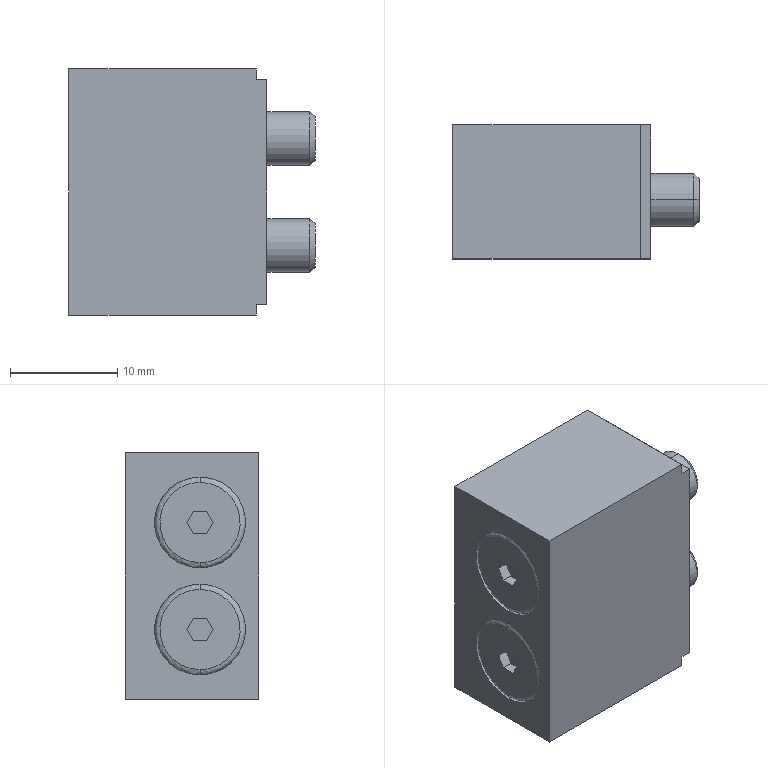Part | SolidWorks | features BaseBody 1 | 1 solid | 44 faces | box 23 x 12.5 x 23 mm | volume 5456 mm3 | plane 28 | cylinder 8 | spline 4 | cone 4 | commonest cylinder face diameters 5 x4 8.5 x4
STEP:
#1=CARTESIAN_POINT('',(-17.5,0.,8.75));
#2=VERTEX_POINT('',#1);
#3=CARTESIAN_POINT('',(-17.5,0.,1.25));
#4=VERTEX_POINT('',#3);
#5=CARTESIAN_POINT('',(-17.5,0.,8.75));
#6=CARTESIAN_POINT('',(-17.5,-7.5,8.75));
#7=CARTESIAN_POINT('',(-17.5,-7.5,1.25));
#8=CARTESIAN_POINT('',(-17.5,0.,1.25));
#9=(BOUNDED_CURVE()B_SPLINE_CURVE(3,(#5,#6,#7,#8),.UNSPECIFIED.,.F.,.F.)B_SPLINE_CURVE_WITH_KNOTS((4,4),(0.,0.5),.UNSPECIFIED.)CURVE()GEOMETRIC_REPRESENTATION_ITEM()RATIONAL_B_SPLINE_CURVE((1.,0.3333,0.3333,1.))REPRESENTATION_ITEM(''));
#10=EDGE_CURVE('',#2,#4,#9,.T.);
#11=ORIENTED_EDGE('',*,*,#10,.T.);
#12=CARTESIAN_POINT('',(-17.,0.,0.75));
#13=VERTEX_POINT('',#12);
#14=CARTESIAN_POINT('',(-17.,0.,1.25));
#15=DIRECTION('',(0.,-1.,0.));
#16=DIRECTION('',(0.,0.,-1.));
#17=AXIS2_PLACEMENT_3D('',#14,#15,#16);
#18=CIRCLE('',#17,0.5);
#19=EDGE_CURVE('',#4,#13,#18,.T.);
#20=ORIENTED_EDGE('',*,*,#19,.T.);
#21=CARTESIAN_POINT('',(-17.,0.,9.25));
#22=VERTEX_POINT('',#21);
#23=CARTESIAN_POINT('',(-17.,0.,5.));
#24=DIRECTION('',(-1.,0.,0.));
#25=DIRECTION('',(0.,0.,-1.));
#26=AXIS2_PLACEMENT_3D('',#23,#24,#25);
#27=CIRCLE('',#26,4.25);
#28=EDGE_CURVE('',#13,#22,#27,.T.);
#29=ORIENTED_EDGE('',*,*,#28,.T.);
#30=CARTESIAN_POINT('',(-17.,0.,8.75));
#31=DIRECTION('',(0.,1.,0.));
#32=DIRECTION('',(0.,0.,1.));
#33=AXIS2_PLACEMENT_3D('',#30,#31,#32);
#34=CIRCLE('',#33,0.5);
#35=EDGE_CURVE('',#2,#22,#34,.T.);
#36=ORIENTED_EDGE('',*,*,#35,.F.);
#37=EDGE_LOOP('',(#11,#20,#29,#36));
#38=FACE_OUTER_BOUND('',#37,.T.);
#39=CARTESIAN_POINT('',(-17.5,0.,1.25));
#40=CARTESIAN_POINT('',(-17.5,-7.5,1.25));
#41=CARTESIAN_POINT('',(-17.5,-7.5,8.75));
#42=CARTESIAN_POINT('',(-17.5,0.,8.75));
#43=CARTESIAN_POINT('',(-17.5,0.,0.9571));
#44=CARTESIAN_POINT('',(-17.5,-8.086,0.9571));
#45=CARTESIAN_POINT('',(-17.5,-8.086,9.043));
#46=CARTESIAN_POINT('',(-17.5,0.,9.043));
#47=CARTESIAN_POINT('',(-17.293,0.,0.75));
#48=CARTESIAN_POINT('',(-17.293,-8.5,0.75));
#49=CARTESIAN_POINT('',(-17.293,-8.5,9.25));
#50=CARTESIAN_POINT('',(-17.293,0.,9.25));
#51=CARTESIAN_POINT('',(-17.,0.,0.75));
#52=CARTESIAN_POINT('',(-17.,-8.5,0.75));
#53=CARTESIAN_POINT('',(-17.,-8.5,9.25));
#54=CARTESIAN_POINT('',(-17.,0.,9.25));
#55=(BOUNDED_SURFACE()B_SPLINE_SURFACE(3,3,((#39,#40,#41,#42),(#43,#44,#45,#46),(#47,#48,#49,#50),(#51,#52,#53,#54)),.UNSPECIFIED.,.F.,.F.,.F.)B_SPLINE_SURFACE_WITH_KNOTS((4,4),(4,4),(0.,1.),(0.,1.),.UNSPECIFIED.)GEOMETRIC_REPRESENTATION_ITEM()RATIONAL_B_SPLINE_SURFACE(((1.,0.3333,0.3333,1.),(0.8047,0.2682,0.2682,0.8047),(0.8047,0.2682,0.2682,0.8047),(1.,0.3333,0.3333,1.)))REPRESENTATION_ITEM('')SURFACE());
#56=ADVANCED_FACE('',(#38),#55,.T.);
#57=CARTESIAN_POINT('',(-17.5,0.,-1.25));
#58=VERTEX_POINT('',#57);
#59=CARTESIAN_POINT('',(-17.5,0.,-8.75));
#60=VERTEX_POINT('',#59);
#61=CARTESIAN_POINT('',(-17.5,0.,-1.25));
#62=CARTESIAN_POINT('',(-17.5,-7.5,-1.25));
#63=CARTESIAN_POINT('',(-17.5,-7.5,-8.75));
#64=CARTESIAN_POINT('',(-17.5,0.,-8.75));
#65=(BOUNDED_CURVE()B_SPLINE_CURVE(3,(#61,#62,#63,#64),.UNSPECIFIED.,.F.,.T.)B_SPLINE_CURVE_WITH_KNOTS((4,4),(0.,0.5),.UNSPECIFIED.)CURVE()GEOMETRIC_REPRESENTATION_ITEM()RATIONAL_B_SPLINE_CURVE((1.,0.3333,0.3333,1.))REPRESENTATION_ITEM(''));
#66=EDGE_CURVE('',#58,#60,#65,.T.);
#67=ORIENTED_EDGE('',*,*,#66,.T.);
#68=CARTESIAN_POINT('',(-17.,0.,-9.25));
#69=VERTEX_POINT('',#68);
#70=CARTESIAN_POINT('',(-17.,0.,-8.75));
#71=DIRECTION('',(0.,-1.,0.));
#72=DIRECTION('',(0.,0.,-1.));
#73=AXIS2_PLACEMENT_3D('',#70,#71,#72);
#74=CIRCLE('',#73,0.5);
#75=EDGE_CURVE('',#60,#69,#74,.T.);
#76=ORIENTED_EDGE('',*,*,#75,.T.);
#77=CARTESIAN_POINT('',(-17.,0.,-0.75));
#78=VERTEX_POINT('',#77);
#79=CARTESIAN_POINT('',(-17.,0.,-5.));
#80=DIRECTION('',(-1.,0.,0.));
#81=DIRECTION('',(0.,0.,-1.));
#82=AXIS2_PLACEMENT_3D('',#79,#80,#81);
#83=CIRCLE('',#82,4.25);
#84=EDGE_CURVE('',#69,#78,#83,.T.);
#85=ORIENTED_EDGE('',*,*,#84,.T.);
#86=CARTESIAN_POINT('',(-17.,0.,-1.25));
#87=DIRECTION('',(0.,1.,0.));
#88=DIRECTION('',(0.,0.,1.));
#89=AXIS2_PLACEMENT_3D('',#86,#87,#88);
#90=CIRCLE('',#89,0.5);
#91=EDGE_CURVE('',#58,#78,#90,.T.);
#92=ORIENTED_EDGE('',*,*,#91,.F.);
#93=EDGE_LOOP('',(#67,#76,#85,#92));
#94=FACE_OUTER_BOUND('',#93,.T.);
#95=CARTESIAN_POINT('',(-17.5,0.,-8.75));
#96=CARTESIAN_POINT('',(-17.5,-7.5,-8.75));
#97=CARTESIAN_POINT('',(-17.5,-7.5,-1.25));
#98=CARTESIAN_POINT('',(-17.5,0.,-1.25));
#99=CARTESIAN_POINT('',(-17.5,0.,-9.043));
#100=CARTESIAN_POINT('',(-17.5,-8.086,-9.043));
#101=CARTESIAN_POINT('',(-17.5,-8.086,-0.9571));
#102=CARTESIAN_POINT('',(-17.5,0.,-0.9571));
#103=CARTESIAN_POINT('',(-17.293,0.,-9.25));
#104=CARTESIAN_POINT('',(-17.293,-8.5,-9.25));
#105=CARTESIAN_POINT('',(-17.293,-8.5,-0.75));
#106=CARTESIAN_POINT('',(-17.293,0.,-0.75));
#107=CARTESIAN_POINT('',(-17.,0.,-9.25));
#108=CARTESIAN_POINT('',(-17.,-8.5,-9.25));
#109=CARTESIAN_POINT('',(-17.,-8.5,-0.75));
#110=CARTESIAN_POINT('',(-17.,0.,-0.75));
#111=(BOUNDED_SURFACE()B_SPLINE_SURFACE(3,3,((#95,#96,#97,#98),(#99,#100,#101,#102),(#103,#104,#105,#106),(#107,#108,#109,#110)),.UNSPECIFIED.,.F.,.F.,.F.)B_SPLINE_SURFACE_WITH_KNOTS((4,4),(4,4),(0.,1.),(0.,1.),.UNSPECIFIED.)GEOMETRIC_REPRESENTATION_ITEM()RATIONAL_B_SPLINE_SURFACE(((1.,0.3333,0.3333,1.),(0.8047,0.2682,0.2682,0.8047),(0.8047,0.2682,0.2682,0.8047),(1.,0.3333,0.3333,1.)))REPRESENTATION_ITEM('')SURFACE());
#112=ADVANCED_FACE('',(#94),#111,.T.);
#113=CARTESIAN_POINT('',(-17.5,0.,0.75));
#114=VERTEX_POINT('',#113);
#115=CARTESIAN_POINT('',(-17.5,0.,9.25));
#116=VERTEX_POINT('',#115);
#117=CARTESIAN_POINT('',(-17.5,0.,5.));
#118=DIRECTION('',(-1.,0.,0.));
#119=DIRECTION('',(0.,0.,-1.));
#120=AXIS2_PLACEMENT_3D('',#117,#118,#119);
#121=CIRCLE('',#120,4.25);
#122=EDGE_CURVE('',#114,#116,#121,.T.);
#123=ORIENTED_EDGE('',*,*,#122,.T.);
#124=CARTESIAN_POINT('',(-50.,0.,9.25));
#125=DIRECTION('',(1.,0.,0.));
#126=VECTOR('',#125,1000.);
#127=LINE('',#124,#126);
#128=EDGE_CURVE('',#116,#22,#127,.T.);
#129=ORIENTED_EDGE('',*,*,#128,.T.);
#130=ORIENTED_EDGE('',*,*,#28,.F.);
#131=CARTESIAN_POINT('',(-50.,0.,0.75));
#132=DIRECTION('',(1.,0.,0.));
#133=VECTOR('',#132,1000.);
#134=LINE('',#131,#133);
#135=EDGE_CURVE('',#114,#13,#134,.T.);
#136=ORIENTED_EDGE('',*,*,#135,.F.);
#137=EDGE_LOOP('',(#123,#129,#130,#136));
#138=FACE_OUTER_BOUND('',#137,.T.);
#139=CARTESIAN_POINT('',(-50.,0.,5.));
#140=DIRECTION('',(1.,0.,0.));
#141=DIRECTION('',(0.,0.,-1.));
#142=AXIS2_PLACEMENT_3D('',#139,#140,#141);
#143=CYLINDRICAL_SURFACE('',#142,4.25);
#144=ADVANCED_FACE('',(#138),#143,.F.);
#145=CARTESIAN_POINT('',(-17.5,0.,-9.25));
#146=VERTEX_POINT('',#145);
#147=CARTESIAN_POINT('',(-17.5,0.,-0.75));
#148=VERTEX_POINT('',#147);
#149=CARTESIAN_POINT('',(-17.5,0.,-5.));
#150=DIRECTION('',(-1.,0.,0.));
#151=DIRECTION('',(0.,0.,-1.));
#152=AXIS2_PLACEMENT_3D('',#149,#150,#151);
#153=CIRCLE('',#152,4.25);
#154=EDGE_CURVE('',#146,#148,#153,.T.);
#155=ORIENTED_EDGE('',*,*,#154,.T.);
#156=CARTESIAN_POINT('',(-50.,0.,-0.75));
#157=DIRECTION('',(1.,0.,0.));
#158=VECTOR('',#157,1000.);
#159=LINE('',#156,#158);
#160=EDGE_CURVE('',#148,#78,#159,.T.);
#161=ORIENTED_EDGE('',*,*,#160,.T.);
#162=ORIENTED_EDGE('',*,*,#84,.F.);
#163=CARTESIAN_POINT('',(-50.,0.,-9.25));
#164=DIRECTION('',(1.,0.,0.));
#165=VECTOR('',#164,1000.);
#166=LINE('',#163,#165);
#167=EDGE_CURVE('',#146,#69,#166,.T.);
#168=ORIENTED_EDGE('',*,*,#167,.F.);
#169=EDGE_LOOP('',(#155,#161,#162,#168));
#170=FACE_OUTER_BOUND('',#169,.T.);
#171=CARTESIAN_POINT('',(-50.,0.,-5.));
#172=DIRECTION('',(1.,0.,0.));
#173=DIRECTION('',(0.,0.,-1.));
#174=AXIS2_PLACEMENT_3D('',#171,#172,#173);
#175=CYLINDRICAL_SURFACE('',#174,4.25);
#176=ADVANCED_FACE('',(#170),#175,.F.);
#177=CARTESIAN_POINT('',(5.01,0.,7.5));
#178=VERTEX_POINT('',#177);
#179=CARTESIAN_POINT('',(5.01,0.,2.5));
#180=VERTEX_POINT('',#179);
#181=CARTESIAN_POINT('',(5.01,0.,5.));
#182=DIRECTION('',(-1.,0.,0.));
#183=DIRECTION('',(0.,0.,1.));
#184=AXIS2_PLACEMENT_3D('',#181,#182,#183);
#185=CIRCLE('',#184,2.5);
#186=EDGE_CURVE('',#178,#180,#185,.T.);
#187=ORIENTED_EDGE('',*,*,#186,.T.);
#188=CARTESIAN_POINT('',(1.,0.,2.5));
#189=VERTEX_POINT('',#188);
#190=CARTESIAN_POINT('',(5.5,0.,2.5));
#191=DIRECTION('',(-1.,0.,0.));
#192=VECTOR('',#191,1000.);
#193=LINE('',#190,#192);
#194=EDGE_CURVE('',#180,#189,#193,.T.);
#195=ORIENTED_EDGE('',*,*,#194,.T.);
#196=CARTESIAN_POINT('',(1.,0.,7.5));
#197=VERTEX_POINT('',#196);
#198=CARTESIAN_POINT('',(1.,0.,5.));
#199=DIRECTION('',(1.,0.,0.));
#200=DIRECTION('',(0.,0.,1.));
#201=AXIS2_PLACEMENT_3D('',#198,#199,#200);
#202=CIRCLE('',#201,2.5);
#203=EDGE_CURVE('',#189,#197,#202,.T.);
#204=ORIENTED_EDGE('',*,*,#203,.T.);
#205=CARTESIAN_POINT('',(5.5,0.,7.5));
#206=DIRECTION('',(-1.,0.,0.));
#207=VECTOR('',#206,1000.);
#208=LINE('',#205,#207);
#209=EDGE_CURVE('',#178,#197,#208,.T.);
#210=ORIENTED_EDGE('',*,*,#209,.F.);
#211=EDGE_LOOP('',(#187,#195,#204,#210));
#212=FACE_OUTER_BOUND('',#211,.T.);
#213=CARTESIAN_POINT('',(5.5,0.,5.));
#214=DIRECTION('',(-1.,0.,0.));
#215=DIRECTION('',(0.,0.,1.));
#216=AXIS2_PLACEMENT_3D('',#213,#214,#215);
#217=CYLINDRICAL_SURFACE('',#216,2.5);
#218=ADVANCED_FACE('',(#212),#217,.T.);
#219=CARTESIAN_POINT('',(5.01,0.,-2.5));
#220=VERTEX_POINT('',#219);
#221=CARTESIAN_POINT('',(5.01,0.,-7.5));
#222=VERTEX_POINT('',#221);
#223=CARTESIAN_POINT('',(5.01,0.,-5.));
#224=DIRECTION('',(-1.,0.,0.));
#225=DIRECTION('',(0.,0.,1.));
#226=AXIS2_PLACEMENT_3D('',#223,#224,#225);
#227=CIRCLE('',#226,2.5);
#228=EDGE_CURVE('',#220,#222,#227,.T.);
#229=ORIENTED_EDGE('',*,*,#228,.T.);
#230=CARTESIAN_POINT('',(1.,0.,-7.5));
#231=VERTEX_POINT('',#230);
#232=CARTESIAN_POINT('',(5.5,0.,-7.5));
#233=DIRECTION('',(-1.,0.,0.));
#234=VECTOR('',#233,1000.);
#235=LINE('',#232,#234);
#236=EDGE_CURVE('',#222,#231,#235,.T.);
#237=ORIENTED_EDGE('',*,*,#236,.T.);
#238=CARTESIAN_POINT('',(1.,0.,-2.5));
#239=VERTEX_POINT('',#238);
#240=CARTESIAN_POINT('',(1.,0.,-5.));
#241=DIRECTION('',(1.,0.,0.));
#242=DIRECTION('',(0.,0.,1.));
#243=AXIS2_PLACEMENT_3D('',#240,#241,#242);
#244=CIRCLE('',#243,2.5);
#245=EDGE_CURVE('',#231,#239,#244,.T.);
#246=ORIENTED_EDGE('',*,*,#245,.T.);
#247=CARTESIAN_POINT('',(5.5,0.,-2.5));
#248=DIRECTION('',(-1.,0.,0.));
#249=VECTOR('',#248,1000.);
#250=LINE('',#247,#249);
#251=EDGE_CURVE('',#220,#239,#250,.T.);
#252=ORIENTED_EDGE('',*,*,#251,.F.);
#253=EDGE_LOOP('',(#229,#237,#246,#252));
#254=FACE_OUTER_BOUND('',#253,.T.);
#255=CARTESIAN_POINT('',(5.5,0.,-5.));
#256=DIRECTION('',(-1.,0.,0.));
#257=DIRECTION('',(0.,0.,1.));
#258=AXIS2_PLACEMENT_3D('',#255,#256,#257);
#259=CYLINDRICAL_SURFACE('',#258,2.5);
#260=ADVANCED_FACE('',(#254),#259,.T.);
#261=CARTESIAN_POINT('',(5.5,0.,7.009));
#262=VERTEX_POINT('',#261);
#263=CARTESIAN_POINT('',(5.5,0.,2.991));
#264=VERTEX_POINT('',#263);
#265=CARTESIAN_POINT('',(5.5,0.,5.));
#266=DIRECTION('',(-1.,0.,0.));
#267=DIRECTION('',(0.,0.,1.));
#268=AXIS2_PLACEMENT_3D('',#265,#266,#267);
#269=CIRCLE('',#268,2.009);
#270=EDGE_CURVE('',#262,#264,#269,.T.);
#271=ORIENTED_EDGE('',*,*,#270,.T.);
#272=CARTESIAN_POINT('',(5.01,0.,2.5));
#273=DIRECTION('',(-0.7071,0.,-0.7071));
#274=VECTOR('',#273,1000.);
#275=LINE('',#272,#274);
#276=EDGE_CURVE('',#264,#180,#275,.T.);
#277=ORIENTED_EDGE('',*,*,#276,.T.);
#278=ORIENTED_EDGE('',*,*,#186,.F.);
#279=CARTESIAN_POINT('',(5.01,0.,7.5));
#280=DIRECTION('',(-0.7071,0.,0.7071));
#281=VECTOR('',#280,1000.);
#282=LINE('',#279,#281);
#283=EDGE_CURVE('',#262,#178,#282,.T.);
#284=ORIENTED_EDGE('',*,*,#283,.F.);
#285=EDGE_LOOP('',(#271,#277,#278,#284));
#286=FACE_OUTER_BOUND('',#285,.T.);
#287=CARTESIAN_POINT('',(5.01,0.,5.));
#288=DIRECTION('',(-1.,0.,0.));
#289=DIRECTION('',(0.,0.,1.));
#290=AXIS2_PLACEMENT_3D('',#287,#288,#289);
#291=CONICAL_SURFACE('',#290,2.5,0.7854);
#292=ADVANCED_FACE('',(#286),#291,.T.);
#293=CARTESIAN_POINT('',(5.5,0.,-2.991));
#294=VERTEX_POINT('',#293);
#295=CARTESIAN_POINT('',(5.5,0.,-7.009));
#296=VERTEX_POINT('',#295);
#297=CARTESIAN_POINT('',(5.5,0.,-5.));
#298=DIRECTION('',(-1.,0.,0.));
#299=DIRECTION('',(0.,0.,1.));
#300=AXIS2_PLACEMENT_3D('',#297,#298,#299);
#301=CIRCLE('',#300,2.009);
#302=EDGE_CURVE('',#294,#296,#301,.T.);
#303=ORIENTED_EDGE('',*,*,#302,.T.);
#304=CARTESIAN_POINT('',(5.01,0.,-7.5));
#305=DIRECTION('',(-0.7071,0.,-0.7071));
#306=VECTOR('',#305,1000.);
#307=LINE('',#304,#306);
#308=EDGE_CURVE('',#296,#222,#307,.T.);
#309=ORIENTED_EDGE('',*,*,#308,.T.);
#310=ORIENTED_EDGE('',*,*,#228,.F.);
#311=CARTESIAN_POINT('',(5.01,0.,-2.5));
#312=DIRECTION('',(-0.7071,0.,0.7071));
#313=VECTOR('',#312,1000.);
#314=LINE('',#311,#313);
#315=EDGE_CURVE('',#294,#220,#314,.T.);
#316=ORIENTED_EDGE('',*,*,#315,.F.);
#317=EDGE_LOOP('',(#303,#309,#310,#316));
#318=FACE_OUTER_BOUND('',#317,.T.);
#319=CARTESIAN_POINT('',(5.01,0.,-5.));
#320=DIRECTION('',(-1.,0.,0.));
#321=DIRECTION('',(0.,0.,1.));
#322=AXIS2_PLACEMENT_3D('',#319,#320,#321);
#323=CONICAL_SURFACE('',#322,2.5,0.7854);
#324=ADVANCED_FACE('',(#318),#323,.T.);
#325=CARTESIAN_POINT('',(0.,-5.5,-11.5));
#326=VERTEX_POINT('',#325);
#327=CARTESIAN_POINT('',(-17.5,-5.5,-11.5));
#328=VERTEX_POINT('',#327);
#329=CARTESIAN_POINT('',(0.,-5.5,-11.5));
#330=DIRECTION('',(-1.,0.,0.));
#331=VECTOR('',#330,1000.);
#332=LINE('',#329,#331);
#333=EDGE_CURVE('',#326,#328,#332,.T.);
#334=ORIENTED_EDGE('',*,*,#333,.F.);
#335=CARTESIAN_POINT('',(0.,-5.5,-10.5));
#336=VERTEX_POINT('',#335);
#337=CARTESIAN_POINT('',(0.,-5.5,-10.5));
#338=DIRECTION('',(0.,0.,1.));
#339=VECTOR('',#338,1000.);
#340=LINE('',#337,#339);
#341=EDGE_CURVE('',#326,#336,#340,.T.);
#342=ORIENTED_EDGE('',*,*,#341,.T.);
#343=CARTESIAN_POINT('',(1.,-5.5,-10.5));
#344=VERTEX_POINT('',#343);
#345=CARTESIAN_POINT('',(1.,-5.5,-10.5));
#346=DIRECTION('',(1.,0.,0.));
#347=VECTOR('',#346,1000.);
#348=LINE('',#345,#347);
#349=EDGE_CURVE('',#336,#344,#348,.T.);
#350=ORIENTED_EDGE('',*,*,#349,.T.);
#351=CARTESIAN_POINT('',(1.,-5.5,10.5));
#352=VERTEX_POINT('',#351);
#353=CARTESIAN_POINT('',(1.,-5.5,0.));
#354=DIRECTION('',(0.,0.,-1.));
#355=VECTOR('',#354,1000.);
#356=LINE('',#353,#355);
#357=EDGE_CURVE('',#352,#344,#356,.T.);
#358=ORIENTED_EDGE('',*,*,#357,.F.);
#359=CARTESIAN_POINT('',(0.,-5.5,10.5));
#360=VERTEX_POINT('',#359);
#361=CARTESIAN_POINT('',(0.,-5.5,10.5));
#362=DIRECTION('',(-1.,0.,0.));
#363=VECTOR('',#362,1000.);
#364=LINE('',#361,#363);
#365=EDGE_CURVE('',#352,#360,#364,.T.);
#366=ORIENTED_EDGE('',*,*,#365,.T.);
#367=CARTESIAN_POINT('',(0.,-5.5,11.5));
#368=VERTEX_POINT('',#367);
#369=CARTESIAN_POINT('',(0.,-5.5,11.5));
#370=DIRECTION('',(0.,0.,1.));
#371=VECTOR('',#370,1000.);
#372=LINE('',#369,#371);
#373=EDGE_CURVE('',#360,#368,#372,.T.);
#374=ORIENTED_EDGE('',*,*,#373,.T.);
#375=CARTESIAN_POINT('',(-17.5,-5.5,11.5));
#376=VERTEX_POINT('',#375);
#377=CARTESIAN_POINT('',(0.,-5.5,11.5));
#378=DIRECTION('',(1.,0.,0.));
#379=VECTOR('',#378,1000.);
#380=LINE('',#377,#379);
#381=EDGE_CURVE('',#376,#368,#380,.T.);
#382=ORIENTED_EDGE('',*,*,#381,.F.);
#383=CARTESIAN_POINT('',(-17.5,-5.5,0.));
#384=DIRECTION('',(0.,0.,1.));
#385=VECTOR('',#384,1000.);
#386=LINE('',#383,#385);
#387=EDGE_CURVE('',#328,#376,#386,.T.);
#388=ORIENTED_EDGE('',*,*,#387,.F.);
#389=EDGE_LOOP('',(#334,#342,#350,#358,#366,#374,#382,#388));
#390=FACE_OUTER_BOUND('',#389,.T.);
#391=CARTESIAN_POINT('',(0.,-5.5,0.));
#392=DIRECTION('',(0.,1.,0.));
#393=DIRECTION('',(0.,0.,1.));
#394=AXIS2_PLACEMENT_3D('',#391,#392,#393);
#395=PLANE('',#394);
#396=ADVANCED_FACE('',(#390),#395,.F.);
#397=CARTESIAN_POINT('',(-17.5,7.,11.5));
#398=VERTEX_POINT('',#397);
#399=CARTESIAN_POINT('',(-17.5,7.,11.5));
#400=DIRECTION('',(0.,-1.,0.));
#401=VECTOR('',#400,1000.);
#402=LINE('',#399,#401);
#403=EDGE_CURVE('',#398,#376,#402,.T.);
#404=ORIENTED_EDGE('',*,*,#403,.F.);
#405=CARTESIAN_POINT('',(-17.5,7.,-11.5));
#406=VERTEX_POINT('',#405);
#407=CARTESIAN_POINT('',(-17.5,7.,-11.5));
#408=DIRECTION('',(0.,0.,1.));
#409=VECTOR('',#408,1000.);
#410=LINE('',#407,#409);
#411=EDGE_CURVE('',#406,#398,#410,.T.);
#412=ORIENTED_EDGE('',*,*,#411,.F.);
#413=CARTESIAN_POINT('',(-17.5,7.,-11.5));
#414=DIRECTION('',(0.,1.,0.));
#415=VECTOR('',#414,1000.);
#416=LINE('',#413,#415);
#417=EDGE_CURVE('',#328,#406,#416,.T.);
#418=ORIENTED_EDGE('',*,*,#417,.F.);
#419=ORIENTED_EDGE('',*,*,#387,.T.);
#420=EDGE_LOOP('',(#404,#412,#418,#419));
#421=FACE_OUTER_BOUND('',#420,.T.);
#422=ORIENTED_EDGE('',*,*,#122,.F.);
#423=CARTESIAN_POINT('',(-17.5,0.,5.));
#424=DIRECTION('',(-1.,0.,0.));
#425=DIRECTION('',(0.,0.,-1.));
#426=AXIS2_PLACEMENT_3D('',#423,#424,#425);
#427=CIRCLE('',#426,4.25);
#428=EDGE_CURVE('',#116,#114,#427,.T.);
#429=ORIENTED_EDGE('',*,*,#428,.F.);
#430=EDGE_LOOP('',(#422,#429));
#431=FACE_BOUND('',#430,.T.);
#432=ORIENTED_EDGE('',*,*,#154,.F.);
#433=CARTESIAN_POINT('',(-17.5,0.,-5.));
#434=DIRECTION('',(-1.,0.,0.));
#435=DIRECTION('',(0.,0.,-1.));
#436=AXIS2_PLACEMENT_3D('',#433,#434,#435);
#437=CIRCLE('',#436,4.25);
#438=EDGE_CURVE('',#148,#146,#437,.T.);
#439=ORIENTED_EDGE('',*,*,#438,.F.);
#440=EDGE_LOOP('',(#432,#439));
#441=FACE_BOUND('',#440,.T.);
#442=CARTESIAN_POINT('',(-17.5,7.,-11.5));
#443=DIRECTION('',(1.,0.,0.));
#444=DIRECTION('',(0.,0.,-1.));
#445=AXIS2_PLACEMENT_3D('',#442,#443,#444);
#446=PLANE('',#445);
#447=ADVANCED_FACE('',(#421,#431,#441),#446,.F.);
#448=ORIENTED_EDGE('',*,*,#417,.T.);
#449=CARTESIAN_POINT('',(0.,7.,-11.5));
#450=VERTEX_POINT('',#449);
#451=CARTESIAN_POINT('',(0.,7.,-11.5));
#452=DIRECTION('',(-1.,0.,0.));
#453=VECTOR('',#452,1000.);
#454=LINE('',#451,#453);
#455=EDGE_CURVE('',#450,#406,#454,.T.);
#456=ORIENTED_EDGE('',*,*,#455,.F.);
#457=CARTESIAN_POINT('',(0.,7.,-11.5));
#458=DIRECTION('',(0.,1.,0.));
#459=VECTOR('',#458,1000.);
#460=LINE('',#457,#459);
#461=EDGE_CURVE('',#326,#450,#460,.T.);
#462=ORIENTED_EDGE('',*,*,#461,.F.);
#463=ORIENTED_EDGE('',*,*,#333,.T.);
#464=EDGE_LOOP('',(#448,#456,#462,#463));
#465=FACE_OUTER_BOUND('',#464,.T.);
#466=CARTESIAN_POINT('',(0.,7.,-11.5));
#467=DIRECTION('',(0.,0.,1.));
#468=DIRECTION('',(1.,0.,0.));
#469=AXIS2_PLACEMENT_3D('',#466,#467,#468);
#470=PLANE('',#469);
#471=ADVANCED_FACE('',(#465),#470,.F.);
#472=CARTESIAN_POINT('',(1.,7.,-10.5));
#473=VERTEX_POINT('',#472);
#474=CARTESIAN_POINT('',(1.,7.,-10.5));
#475=DIRECTION('',(0.,-1.,0.));
#476=VECTOR('',#475,1000.);
#477=LINE('',#474,#476);
#478=EDGE_CURVE('',#473,#344,#477,.T.);
#479=ORIENTED_EDGE('',*,*,#478,.F.);
#480=CARTESIAN_POINT('',(1.,7.,10.5));
#481=VERTEX_POINT('',#480);
#482=CARTESIAN_POINT('',(1.,7.,10.5));
#483=DIRECTION('',(0.,0.,-1.));
#484=VECTOR('',#483,1000.);
#485=LINE('',#482,#484);
#486=EDGE_CURVE('',#481,#473,#485,.T.);
#487=ORIENTED_EDGE('',*,*,#486,.F.);
#488=CARTESIAN_POINT('',(1.,7.,10.5));
#489=DIRECTION('',(0.,1.,0.));
#490=VECTOR('',#489,1000.);
#491=LINE('',#488,#490);
#492=EDGE_CURVE('',#352,#481,#491,.T.);
#493=ORIENTED_EDGE('',*,*,#492,.F.);
#494=ORIENTED_EDGE('',*,*,#357,.T.);
#495=EDGE_LOOP('',(#479,#487,#493,#494));
#496=FACE_OUTER_BOUND('',#495,.T.);
#497=CARTESIAN_POINT('',(1.,0.,5.));
#498=DIRECTION('',(1.,0.,0.));
#499=DIRECTION('',(0.,0.,1.));
#500=AXIS2_PLACEMENT_3D('',#497,#498,#499);
#501=CIRCLE('',#500,2.5);
#502=EDGE_CURVE('',#197,#189,#501,.T.);
#503=ORIENTED_EDGE('',*,*,#502,.F.);
#504=ORIENTED_EDGE('',*,*,#203,.F.);
#505=EDGE_LOOP('',(#503,#504));
#506=FACE_BOUND('',#505,.T.);
#507=CARTESIAN_POINT('',(1.,0.,-5.));
#508=DIRECTION('',(1.,0.,0.));
#509=DIRECTION('',(0.,0.,1.));
#510=AXIS2_PLACEMENT_3D('',#507,#508,#509);
#511=CIRCLE('',#510,2.5);
#512=EDGE_CURVE('',#239,#231,#511,.T.);
#513=ORIENTED_EDGE('',*,*,#512,.F.);
#514=ORIENTED_EDGE('',*,*,#245,.F.);
#515=EDGE_LOOP('',(#513,#514));
#516=FACE_BOUND('',#515,.T.);
#517=CARTESIAN_POINT('',(1.,7.,10.5));
#518=DIRECTION('',(-1.,0.,0.));
#519=DIRECTION('',(0.,0.,1.));
#520=AXIS2_PLACEMENT_3D('',#517,#518,#519);
#521=PLANE('',#520);
#522=ADVANCED_FACE('',(#496,#506,#516),#521,.F.);
#523=CARTESIAN_POINT('',(0.,7.,11.5));
#524=VERTEX_POINT('',#523);
#525=CARTESIAN_POINT('',(0.,7.,11.5));
#526=DIRECTION('',(0.,-1.,0.));
#527=VECTOR('',#526,1000.);
#528=LINE('',#525,#527);
#529=EDGE_CURVE('',#524,#368,#528,.T.);
#530=ORIENTED_EDGE('',*,*,#529,.F.);
#531=CARTESIAN_POINT('',(-17.5,7.,11.5));
#532=DIRECTION('',(1.,0.,0.));
#533=VECTOR('',#532,1000.);
#534=LINE('',#531,#533);
#535=EDGE_CURVE('',#398,#524,#534,.T.);
#536=ORIENTED_EDGE('',*,*,#535,.F.);
#537=ORIENTED_EDGE('',*,*,#403,.T.);
#538=ORIENTED_EDGE('',*,*,#381,.T.);
#539=EDGE_LOOP('',(#530,#536,#537,#538));
#540=FACE_OUTER_BOUND('',#539,.T.);
#541=CARTESIAN_POINT('',(-17.5,7.,11.5));
#542=DIRECTION('',(0.,0.,-1.));
#543=DIRECTION('',(-1.,0.,0.));
#544=AXIS2_PLACEMENT_3D('',#541,#542,#543);
#545=PLANE('',#544);
#546=ADVANCED_FACE('',(#540),#545,.F.);
#547=CARTESIAN_POINT('',(0.,7.,-10.5));
#548=VERTEX_POINT('',#547);
#549=CARTESIAN_POINT('',(0.,7.,0.));
#550=DIRECTION('',(0.,0.,-1.));
#551=VECTOR('',#550,1000.);
#552=LINE('',#549,#551);
#553=EDGE_CURVE('',#548,#450,#552,.T.);
#554=ORIENTED_EDGE('',*,*,#553,.T.);
#555=ORIENTED_EDGE('',*,*,#455,.T.);
#556=ORIENTED_EDGE('',*,*,#411,.T.);
#557=ORIENTED_EDGE('',*,*,#535,.T.);
#558=CARTESIAN_POINT('',(0.,7.,10.5));
#559=VERTEX_POINT('',#558);
#560=CARTESIAN_POINT('',(0.,7.,0.));
#561=DIRECTION('',(0.,0.,-1.));
#562=VECTOR('',#561,1000.);
#563=LINE('',#560,#562);
#564=EDGE_CURVE('',#524,#559,#563,.T.);
#565=ORIENTED_EDGE('',*,*,#564,.T.);
#566=CARTESIAN_POINT('',(0.,7.,10.5));
#567=DIRECTION('',(1.,0.,0.));
#568=VECTOR('',#567,1000.);
#569=LINE('',#566,#568);
#570=EDGE_CURVE('',#559,#481,#569,.T.);
#571=ORIENTED_EDGE('',*,*,#570,.T.);
#572=ORIENTED_EDGE('',*,*,#486,.T.);
#573=CARTESIAN_POINT('',(0.,7.,-10.5));
#574=DIRECTION('',(-1.,0.,0.));
#575=VECTOR('',#574,1000.);
#576=LINE('',#573,#575);
#577=EDGE_CURVE('',#473,#548,#576,.T.);
#578=ORIENTED_EDGE('',*,*,#577,.T.);
#579=EDGE_LOOP('',(#554,#555,#556,#557,#565,#571,#572,#578));
#580=FACE_OUTER_BOUND('',#579,.T.);
#581=CARTESIAN_POINT('',(0.,7.,0.));
#582=DIRECTION('',(0.,1.,0.));
#583=DIRECTION('',(0.,0.,1.));
#584=AXIS2_PLACEMENT_3D('',#581,#582,#583);
#585=PLANE('',#584);
#586=ADVANCED_FACE('',(#580),#585,.T.);
#587=ORIENTED_EDGE('',*,*,#128,.F.);
#588=ORIENTED_EDGE('',*,*,#428,.T.);
#589=ORIENTED_EDGE('',*,*,#135,.T.);
#590=CARTESIAN_POINT('',(-17.,0.,5.));
#591=DIRECTION('',(-1.,0.,0.));
#592=DIRECTION('',(0.,0.,-1.));
#593=AXIS2_PLACEMENT_3D('',#590,#591,#592);
#594=CIRCLE('',#593,4.25);
#595=EDGE_CURVE('',#22,#13,#594,.T.);
#596=ORIENTED_EDGE('',*,*,#595,.F.);
#597=EDGE_LOOP('',(#587,#588,#589,#596));
#598=FACE_OUTER_BOUND('',#597,.T.);
#599=CARTESIAN_POINT('',(-50.,0.,5.));
#600=DIRECTION('',(1.,0.,0.));
#601=DIRECTION('',(0.,0.,-1.));
#602=AXIS2_PLACEMENT_3D('',#599,#600,#601);
#603=CYLINDRICAL_SURFACE('',#602,4.25);
#604=ADVANCED_FACE('',(#598),#603,.F.);
#605=ORIENTED_EDGE('',*,*,#160,.F.);
#606=ORIENTED_EDGE('',*,*,#438,.T.);
#607=ORIENTED_EDGE('',*,*,#167,.T.);
#608=CARTESIAN_POINT('',(-17.,0.,-5.));
#609=DIRECTION('',(-1.,0.,0.));
#610=DIRECTION('',(0.,0.,-1.));
#611=AXIS2_PLACEMENT_3D('',#608,#609,#610);
#612=CIRCLE('',#611,4.25);
#613=EDGE_CURVE('',#78,#69,#612,.T.);
#614=ORIENTED_EDGE('',*,*,#613,.F.);
#615=EDGE_LOOP('',(#605,#606,#607,#614));
#616=FACE_OUTER_BOUND('',#615,.T.);
#617=CARTESIAN_POINT('',(-50.,0.,-5.));
#618=DIRECTION('',(1.,0.,0.));
#619=DIRECTION('',(0.,0.,-1.));
#620=AXIS2_PLACEMENT_3D('',#617,#618,#619);
#621=CYLINDRICAL_SURFACE('',#620,4.25);
#622=ADVANCED_FACE('',(#616),#621,.F.);
#623=ORIENTED_EDGE('',*,*,#461,.T.);
#624=ORIENTED_EDGE('',*,*,#553,.F.);
#625=CARTESIAN_POINT('',(0.,7.,-10.5));
#626=DIRECTION('',(0.,1.,0.));
#627=VECTOR('',#626,1000.);
#628=LINE('',#625,#627);
#629=EDGE_CURVE('',#336,#548,#628,.T.);
#630=ORIENTED_EDGE('',*,*,#629,.F.);
#631=ORIENTED_EDGE('',*,*,#341,.F.);
#632=EDGE_LOOP('',(#623,#624,#630,#631));
#633=FACE_OUTER_BOUND('',#632,.T.);
#634=CARTESIAN_POINT('',(0.,7.,-10.5));
#635=DIRECTION('',(-1.,0.,0.));
#636=DIRECTION('',(0.,0.,1.));
#637=AXIS2_PLACEMENT_3D('',#634,#635,#636);
#638=PLANE('',#637);
#639=ADVANCED_FACE('',(#633),#638,.F.);
#640=ORIENTED_EDGE('',*,*,#629,.T.);
#641=ORIENTED_EDGE('',*,*,#577,.F.);
#642=ORIENTED_EDGE('',*,*,#478,.T.);
#643=ORIENTED_EDGE('',*,*,#349,.F.);
#644=EDGE_LOOP('',(#640,#641,#642,#643));
#645=FACE_OUTER_BOUND('',#644,.T.);
#646=CARTESIAN_POINT('',(1.,7.,-10.5));
#647=DIRECTION('',(0.,0.,1.));
#648=DIRECTION('',(1.,0.,0.));
#649=AXIS2_PLACEMENT_3D('',#646,#647,#648);
#650=PLANE('',#649);
#651=ADVANCED_FACE('',(#645),#650,.F.);
#652=ORIENTED_EDGE('',*,*,#492,.T.);
#653=ORIENTED_EDGE('',*,*,#570,.F.);
#654=CARTESIAN_POINT('',(0.,7.,10.5));
#655=DIRECTION('',(0.,1.,0.));
#656=VECTOR('',#655,1000.);
#657=LINE('',#654,#656);
#658=EDGE_CURVE('',#360,#559,#657,.T.);
#659=ORIENTED_EDGE('',*,*,#658,.F.);
#660=ORIENTED_EDGE('',*,*,#365,.F.);
#661=EDGE_LOOP('',(#652,#653,#659,#660));
#662=FACE_OUTER_BOUND('',#661,.T.);
#663=CARTESIAN_POINT('',(0.,7.,10.5));
#664=DIRECTION('',(0.,0.,-1.));
#665=DIRECTION('',(-1.,0.,0.));
#666=AXIS2_PLACEMENT_3D('',#663,#664,#665);
#667=PLANE('',#666);
#668=ADVANCED_FACE('',(#662),#667,.F.);
#669=ORIENTED_EDGE('',*,*,#194,.F.);
#670=CARTESIAN_POINT('',(5.01,0.,5.));
#671=DIRECTION('',(-1.,0.,0.));
#672=DIRECTION('',(0.,0.,1.));
#673=AXIS2_PLACEMENT_3D('',#670,#671,#672);
#674=CIRCLE('',#673,2.5);
#675=EDGE_CURVE('',#180,#178,#674,.T.);
#676=ORIENTED_EDGE('',*,*,#675,.T.);
#677=ORIENTED_EDGE('',*,*,#209,.T.);
#678=ORIENTED_EDGE('',*,*,#502,.T.);
#679=EDGE_LOOP('',(#669,#676,#677,#678));
#680=FACE_OUTER_BOUND('',#679,.T.);
#681=CARTESIAN_POINT('',(5.5,0.,5.));
#682=DIRECTION('',(-1.,0.,0.));
#683=DIRECTION('',(0.,0.,1.));
#684=AXIS2_PLACEMENT_3D('',#681,#682,#683);
#685=CYLINDRICAL_SURFACE('',#684,2.5);
#686=ADVANCED_FACE('',(#680),#685,.T.);
#687=ORIENTED_EDGE('',*,*,#236,.F.);
#688=CARTESIAN_POINT('',(5.01,0.,-5.));
#689=DIRECTION('',(-1.,0.,0.));
#690=DIRECTION('',(0.,0.,1.));
#691=AXIS2_PLACEMENT_3D('',#688,#689,#690);
#692=CIRCLE('',#691,2.5);
#693=EDGE_CURVE('',#222,#220,#692,.T.);
#694=ORIENTED_EDGE('',*,*,#693,.T.);
#695=ORIENTED_EDGE('',*,*,#251,.T.);
#696=ORIENTED_EDGE('',*,*,#512,.T.);
#697=EDGE_LOOP('',(#687,#694,#695,#696));
#698=FACE_OUTER_BOUND('',#697,.T.);
#699=CARTESIAN_POINT('',(5.5,0.,-5.));
#700=DIRECTION('',(-1.,0.,0.));
#701=DIRECTION('',(0.,0.,1.));
#702=AXIS2_PLACEMENT_3D('',#699,#700,#701);
#703=CYLINDRICAL_SURFACE('',#702,2.5);
#704=ADVANCED_FACE('',(#698),#703,.T.);
#705=ORIENTED_EDGE('',*,*,#658,.T.);
#706=ORIENTED_EDGE('',*,*,#564,.F.);
#707=ORIENTED_EDGE('',*,*,#529,.T.);
#708=ORIENTED_EDGE('',*,*,#373,.F.);
#709=EDGE_LOOP('',(#705,#706,#707,#708));
#710=FACE_OUTER_BOUND('',#709,.T.);
#711=CARTESIAN_POINT('',(0.,7.,11.5));
#712=DIRECTION('',(-1.,0.,0.));
#713=DIRECTION('',(0.,0.,1.));
#714=AXIS2_PLACEMENT_3D('',#711,#712,#713);
#715=PLANE('',#714);
#716=ADVANCED_FACE('',(#710),#715,.F.);
#717=ORIENTED_EDGE('',*,*,#19,.F.);
#718=CARTESIAN_POINT('',(-17.5,0.,1.25));
#719=CARTESIAN_POINT('',(-17.5,7.5,1.25));
#720=CARTESIAN_POINT('',(-17.5,7.5,8.75));
#721=CARTESIAN_POINT('',(-17.5,0.,8.75));
#722=(BOUNDED_CURVE()B_SPLINE_CURVE(3,(#718,#719,#720,#721),.UNSPECIFIED.,.F.,.F.)B_SPLINE_CURVE_WITH_KNOTS((4,4),(0.5,1.),.UNSPECIFIED.)CURVE()GEOMETRIC_REPRESENTATION_ITEM()RATIONAL_B_SPLINE_CURVE((1.,0.3333,0.3333,1.))REPRESENTATION_ITEM(''));
#723=EDGE_CURVE('',#4,#2,#722,.T.);
#724=ORIENTED_EDGE('',*,*,#723,.T.);
#725=ORIENTED_EDGE('',*,*,#35,.T.);
#726=ORIENTED_EDGE('',*,*,#595,.T.);
#727=EDGE_LOOP('',(#717,#724,#725,#726));
#728=FACE_OUTER_BOUND('',#727,.T.);
#729=CARTESIAN_POINT('',(-17.5,0.,8.75));
#730=CARTESIAN_POINT('',(-17.5,7.5,8.75));
#731=CARTESIAN_POINT('',(-17.5,7.5,1.25));
#732=CARTESIAN_POINT('',(-17.5,0.,1.25));
#733=CARTESIAN_POINT('',(-17.5,0.,9.043));
#734=CARTESIAN_POINT('',(-17.5,8.086,9.043));
#735=CARTESIAN_POINT('',(-17.5,8.086,0.9571));
#736=CARTESIAN_POINT('',(-17.5,0.,0.9571));
#737=CARTESIAN_POINT('',(-17.293,0.,9.25));
#738=CARTESIAN_POINT('',(-17.293,8.5,9.25));
#739=CARTESIAN_POINT('',(-17.293,8.5,0.75));
#740=CARTESIAN_POINT('',(-17.293,0.,0.75));
#741=CARTESIAN_POINT('',(-17.,0.,9.25));
#742=CARTESIAN_POINT('',(-17.,8.5,9.25));
#743=CARTESIAN_POINT('',(-17.,8.5,0.75));
#744=CARTESIAN_POINT('',(-17.,0.,0.75));
#745=(BOUNDED_SURFACE()B_SPLINE_SURFACE(3,3,((#729,#730,#731,#732),(#733,#734,#735,#736),(#737,#738,#739,#740),(#741,#742,#743,#744)),.UNSPECIFIED.,.F.,.F.,.F.)B_SPLINE_SURFACE_WITH_KNOTS((4,4),(4,4),(0.,1.),(0.,1.),.UNSPECIFIED.)GEOMETRIC_REPRESENTATION_ITEM()RATIONAL_B_SPLINE_SURFACE(((1.,0.3333,0.3333,1.),(0.8047,0.2682,0.2682,0.8047),(0.8047,0.2682,0.2682,0.8047),(1.,0.3333,0.3333,1.)))REPRESENTATION_ITEM('')SURFACE());
#746=ADVANCED_FACE('',(#728),#745,.T.);
#747=ORIENTED_EDGE('',*,*,#75,.F.);
#748=CARTESIAN_POINT('',(-17.5,0.,-8.75));
#749=CARTESIAN_POINT('',(-17.5,7.5,-8.75));
#750=CARTESIAN_POINT('',(-17.5,7.5,-1.25));
#751=CARTESIAN_POINT('',(-17.5,0.,-1.25));
#752=(BOUNDED_CURVE()B_SPLINE_CURVE(3,(#748,#749,#750,#751),.UNSPECIFIED.,.F.,.T.)B_SPLINE_CURVE_WITH_KNOTS((4,4),(0.5,1.),.UNSPECIFIED.)CURVE()GEOMETRIC_REPRESENTATION_ITEM()RATIONAL_B_SPLINE_CURVE((1.,0.3333,0.3333,1.))REPRESENTATION_ITEM(''));
#753=EDGE_CURVE('',#60,#58,#752,.T.);
#754=ORIENTED_EDGE('',*,*,#753,.T.);
#755=ORIENTED_EDGE('',*,*,#91,.T.);
#756=ORIENTED_EDGE('',*,*,#613,.T.);
#757=EDGE_LOOP('',(#747,#754,#755,#756));
#758=FACE_OUTER_BOUND('',#757,.T.);
#759=CARTESIAN_POINT('',(-17.5,0.,-1.25));
#760=CARTESIAN_POINT('',(-17.5,7.5,-1.25));
#761=CARTESIAN_POINT('',(-17.5,7.5,-8.75));
#762=CARTESIAN_POINT('',(-17.5,0.,-8.75));
#763=CARTESIAN_POINT('',(-17.5,0.,-0.9571));
#764=CARTESIAN_POINT('',(-17.5,8.086,-0.9571));
#765=CARTESIAN_POINT('',(-17.5,8.086,-9.043));
#766=CARTESIAN_POINT('',(-17.5,0.,-9.043));
#767=CARTESIAN_POINT('',(-17.293,0.,-0.75));
#768=CARTESIAN_POINT('',(-17.293,8.5,-0.75));
#769=CARTESIAN_POINT('',(-17.293,8.5,-9.25));
#770=CARTESIAN_POINT('',(-17.293,0.,-9.25));
#771=CARTESIAN_POINT('',(-17.,0.,-0.75));
#772=CARTESIAN_POINT('',(-17.,8.5,-0.75));
#773=CARTESIAN_POINT('',(-17.,8.5,-9.25));
#774=CARTESIAN_POINT('',(-17.,0.,-9.25));
#775=(BOUNDED_SURFACE()B_SPLINE_SURFACE(3,3,((#759,#760,#761,#762),(#763,#764,#765,#766),(#767,#768,#769,#770),(#771,#772,#773,#774)),.UNSPECIFIED.,.F.,.F.,.F.)B_SPLINE_SURFACE_WITH_KNOTS((4,4),(4,4),(0.,1.),(0.,1.),.UNSPECIFIED.)GEOMETRIC_REPRESENTATION_ITEM()RATIONAL_B_SPLINE_SURFACE(((1.,0.3333,0.3333,1.),(0.8047,0.2682,0.2682,0.8047),(0.8047,0.2682,0.2682,0.8047),(1.,0.3333,0.3333,1.)))REPRESENTATION_ITEM('')SURFACE());
#776=ADVANCED_FACE('',(#758),#775,.T.);
#777=ORIENTED_EDGE('',*,*,#276,.F.);
#778=CARTESIAN_POINT('',(5.5,0.,5.));
#779=DIRECTION('',(-1.,0.,0.));
#780=DIRECTION('',(0.,0.,1.));
#781=AXIS2_PLACEMENT_3D('',#778,#779,#780);
#782=CIRCLE('',#781,2.009);
#783=EDGE_CURVE('',#264,#262,#782,.T.);
#784=ORIENTED_EDGE('',*,*,#783,.T.);
#785=ORIENTED_EDGE('',*,*,#283,.T.);
#786=ORIENTED_EDGE('',*,*,#675,.F.);
#787=EDGE_LOOP('',(#777,#784,#785,#786));
#788=FACE_OUTER_BOUND('',#787,.T.);
#789=CARTESIAN_POINT('',(5.01,0.,5.));
#790=DIRECTION('',(-1.,0.,0.));
#791=DIRECTION('',(0.,0.,1.));
#792=AXIS2_PLACEMENT_3D('',#789,#790,#791);
#793=CONICAL_SURFACE('',#792,2.5,0.7854);
#794=ADVANCED_FACE('',(#788),#793,.T.);
#795=ORIENTED_EDGE('',*,*,#308,.F.);
#796=CARTESIAN_POINT('',(5.5,0.,-5.));
#797=DIRECTION('',(-1.,0.,0.));
#798=DIRECTION('',(0.,0.,1.));
#799=AXIS2_PLACEMENT_3D('',#796,#797,#798);
#800=CIRCLE('',#799,2.009);
#801=EDGE_CURVE('',#296,#294,#800,.T.);
#802=ORIENTED_EDGE('',*,*,#801,.T.);
#803=ORIENTED_EDGE('',*,*,#315,.T.);
#804=ORIENTED_EDGE('',*,*,#693,.F.);
#805=EDGE_LOOP('',(#795,#802,#803,#804));
#806=FACE_OUTER_BOUND('',#805,.T.);
#807=CARTESIAN_POINT('',(5.01,0.,-5.));
#808=DIRECTION('',(-1.,0.,0.));
#809=DIRECTION('',(0.,0.,1.));
#810=AXIS2_PLACEMENT_3D('',#807,#808,#809);
#811=CONICAL_SURFACE('',#810,2.5,0.7854);
#812=ADVANCED_FACE('',(#806),#811,.T.);
#813=CARTESIAN_POINT('',(-17.5,-1.227,5.));
#814=VERTEX_POINT('',#813);
#815=CARTESIAN_POINT('',(-17.5,-0.6134,6.062));
#816=VERTEX_POINT('',#815);
#817=CARTESIAN_POINT('',(-17.5,-1.227,5.));
#818=DIRECTION('',(0.,0.5,0.866));
#819=VECTOR('',#818,1000.);
#820=LINE('',#817,#819);
#821=EDGE_CURVE('',#814,#816,#820,.T.);
#822=ORIENTED_EDGE('',*,*,#821,.F.);
#823=CARTESIAN_POINT('',(-17.5,-0.6134,3.938));
#824=VERTEX_POINT('',#823);
#825=CARTESIAN_POINT('',(-17.5,-0.6134,3.938));
#826=DIRECTION('',(0.,-0.5,0.866));
#827=VECTOR('',#826,1000.);
#828=LINE('',#825,#827);
#829=EDGE_CURVE('',#824,#814,#828,.T.);
#830=ORIENTED_EDGE('',*,*,#829,.F.);
#831=CARTESIAN_POINT('',(-17.5,0.6134,3.938));
#832=VERTEX_POINT('',#831);
#833=CARTESIAN_POINT('',(-17.5,7.,3.938));
#834=DIRECTION('',(0.,-1.,0.));
#835=VECTOR('',#834,1000.);
#836=LINE('',#833,#835);
#837=EDGE_CURVE('',#832,#824,#836,.T.);
#838=ORIENTED_EDGE('',*,*,#837,.F.);
#839=CARTESIAN_POINT('',(-17.5,1.227,5.));
#840=VERTEX_POINT('',#839);
#841=CARTESIAN_POINT('',(-17.5,1.227,5.));
#842=DIRECTION('',(0.,-0.5,-0.866));
#843=VECTOR('',#842,1000.);
#844=LINE('',#841,#843);
#845=EDGE_CURVE('',#840,#832,#844,.T.);
#846=ORIENTED_EDGE('',*,*,#845,.F.);
#847=CARTESIAN_POINT('',(-17.5,0.6134,6.062));
#848=VERTEX_POINT('',#847);
#849=CARTESIAN_POINT('',(-17.5,0.6134,6.063));
#850=DIRECTION('',(0.,0.5,-0.866));
#851=VECTOR('',#850,1000.);
#852=LINE('',#849,#851);
#853=EDGE_CURVE('',#848,#840,#852,.T.);
#854=ORIENTED_EDGE('',*,*,#853,.F.);
#855=CARTESIAN_POINT('',(-17.5,7.,6.063));
#856=DIRECTION('',(0.,1.,0.));
#857=VECTOR('',#856,1000.);
#858=LINE('',#855,#857);
#859=EDGE_CURVE('',#816,#848,#858,.T.);
#860=ORIENTED_EDGE('',*,*,#859,.F.);
#861=EDGE_LOOP('',(#822,#830,#838,#846,#854,#860));
#862=FACE_BOUND('',#861,.T.);
#863=ORIENTED_EDGE('',*,*,#10,.F.);
#864=ORIENTED_EDGE('',*,*,#723,.F.);
#865=EDGE_LOOP('',(#863,#864));
#866=FACE_OUTER_BOUND('',#865,.T.);
#867=CARTESIAN_POINT('',(-17.5,7.,-11.5));
#868=DIRECTION('',(1.,0.,0.));
#869=DIRECTION('',(0.,0.,-1.));
#870=AXIS2_PLACEMENT_3D('',#867,#868,#869);
#871=PLANE('',#870);
#872=ADVANCED_FACE('',(#862,#866),#871,.F.);
#873=CARTESIAN_POINT('',(-17.5,-1.227,-5.));
#874=VERTEX_POINT('',#873);
#875=CARTESIAN_POINT('',(-17.5,-0.6134,-3.938));
#876=VERTEX_POINT('',#875);
#877=CARTESIAN_POINT('',(-17.5,-1.227,-5.));
#878=DIRECTION('',(0.,0.5,0.866));
#879=VECTOR('',#878,1000.);
#880=LINE('',#877,#879);
#881=EDGE_CURVE('',#874,#876,#880,.T.);
#882=ORIENTED_EDGE('',*,*,#881,.F.);
#883=CARTESIAN_POINT('',(-17.5,-0.6134,-6.062));
#884=VERTEX_POINT('',#883);
#885=CARTESIAN_POINT('',(-17.5,-0.6134,-6.062));
#886=DIRECTION('',(0.,-0.5,0.866));
#887=VECTOR('',#886,1000.);
#888=LINE('',#885,#887);
#889=EDGE_CURVE('',#884,#874,#888,.T.);
#890=ORIENTED_EDGE('',*,*,#889,.F.);
#891=CARTESIAN_POINT('',(-17.5,0.6134,-6.062));
#892=VERTEX_POINT('',#891);
#893=CARTESIAN_POINT('',(-17.5,7.,-6.062));
#894=DIRECTION('',(0.,-1.,0.));
#895=VECTOR('',#894,1000.);
#896=LINE('',#893,#895);
#897=EDGE_CURVE('',#892,#884,#896,.T.);
#898=ORIENTED_EDGE('',*,*,#897,.F.);
#899=CARTESIAN_POINT('',(-17.5,1.227,-5.));
#900=VERTEX_POINT('',#899);
#901=CARTESIAN_POINT('',(-17.5,1.227,-5.));
#902=DIRECTION('',(0.,-0.5,-0.866));
#903=VECTOR('',#902,1000.);
#904=LINE('',#901,#903);
#905=EDGE_CURVE('',#900,#892,#904,.T.);
#906=ORIENTED_EDGE('',*,*,#905,.F.);
#907=CARTESIAN_POINT('',(-17.5,0.6134,-3.938));
#908=VERTEX_POINT('',#907);
#909=CARTESIAN_POINT('',(-17.5,0.6134,-3.938));
#910=DIRECTION('',(0.,0.5,-0.866));
#911=VECTOR('',#910,1000.);
#912=LINE('',#909,#911);
#913=EDGE_CURVE('',#908,#900,#912,.T.);
#914=ORIENTED_EDGE('',*,*,#913,.F.);
#915=CARTESIAN_POINT('',(-17.5,7.,-3.938));
#916=DIRECTION('',(0.,1.,0.));
#917=VECTOR('',#916,1000.);
#918=LINE('',#915,#917);
#919=EDGE_CURVE('',#876,#908,#918,.T.);
#920=ORIENTED_EDGE('',*,*,#919,.F.);
#921=EDGE_LOOP('',(#882,#890,#898,#906,#914,#920));
#922=FACE_BOUND('',#921,.T.);
#923=ORIENTED_EDGE('',*,*,#66,.F.);
#924=ORIENTED_EDGE('',*,*,#753,.F.);
#925=EDGE_LOOP('',(#923,#924));
#926=FACE_OUTER_BOUND('',#925,.T.);
#927=CARTESIAN_POINT('',(-17.5,7.,-11.5));
#928=DIRECTION('',(1.,0.,0.));
#929=DIRECTION('',(0.,0.,-1.));
#930=AXIS2_PLACEMENT_3D('',#927,#928,#929);
#931=PLANE('',#930);
#932=ADVANCED_FACE('',(#922,#926),#931,.F.);
#933=ORIENTED_EDGE('',*,*,#270,.F.);
#934=ORIENTED_EDGE('',*,*,#783,.F.);
#935=EDGE_LOOP('',(#933,#934));
#936=FACE_OUTER_BOUND('',#935,.T.);
#937=CARTESIAN_POINT('',(5.5,0.,2.99));
#938=DIRECTION('',(-1.,0.,0.));
#939=DIRECTION('',(0.,0.,1.));
#940=AXIS2_PLACEMENT_3D('',#937,#938,#939);
#941=PLANE('',#940);
#942=ADVANCED_FACE('',(#936),#941,.F.);
#943=ORIENTED_EDGE('',*,*,#302,.F.);
#944=ORIENTED_EDGE('',*,*,#801,.F.);
#945=EDGE_LOOP('',(#943,#944));
#946=FACE_OUTER_BOUND('',#945,.T.);
#947=CARTESIAN_POINT('',(5.5,0.,-7.01));
#948=DIRECTION('',(-1.,0.,0.));
#949=DIRECTION('',(0.,0.,1.));
#950=AXIS2_PLACEMENT_3D('',#947,#948,#949);
#951=PLANE('',#950);
#952=ADVANCED_FACE('',(#946),#951,.F.);
#953=CARTESIAN_POINT('',(-16.5,0.6134,6.062));
#954=VERTEX_POINT('',#953);
#955=CARTESIAN_POINT('',(-16.5,-0.6134,6.062));
#956=VERTEX_POINT('',#955);
#957=CARTESIAN_POINT('',(-16.5,0.6134,6.062));
#958=DIRECTION('',(0.,-1.,0.));
#959=VECTOR('',#958,1000.);
#960=LINE('',#957,#959);
#961=EDGE_CURVE('',#954,#956,#960,.T.);
#962=ORIENTED_EDGE('',*,*,#961,.T.);
#963=CARTESIAN_POINT('',(-16.5,-0.6134,6.062));
#964=DIRECTION('',(-1.,0.,0.));
#965=VECTOR('',#964,1000.);
#966=LINE('',#963,#965);
#967=EDGE_CURVE('',#956,#816,#966,.T.);
#968=ORIENTED_EDGE('',*,*,#967,.T.);
#969=ORIENTED_EDGE('',*,*,#859,.T.);
#970=CARTESIAN_POINT('',(-16.5,0.6134,6.062));
#971=DIRECTION('',(1.,0.,0.));
#972=VECTOR('',#971,1000.);
#973=LINE('',#970,#972);
#974=EDGE_CURVE('',#848,#954,#973,.T.);
#975=ORIENTED_EDGE('',*,*,#974,.T.);
#976=EDGE_LOOP('',(#962,#968,#969,#975));
#977=FACE_OUTER_BOUND('',#976,.T.);
#978=CARTESIAN_POINT('',(-16.5,0.6134,6.062));
#979=DIRECTION('',(0.,0.,-1.));
#980=DIRECTION('',(-1.,0.,0.));
#981=AXIS2_PLACEMENT_3D('',#978,#979,#980);
#982=PLANE('',#981);
#983=ADVANCED_FACE('',(#977),#982,.T.);
#984=CARTESIAN_POINT('',(-16.5,-1.227,5.));
#985=VERTEX_POINT('',#984);
#986=CARTESIAN_POINT('',(-16.5,-0.6134,6.062));
#987=DIRECTION('',(0.,-0.5,-0.866));
#988=VECTOR('',#987,1000.);
#989=LINE('',#986,#988);
#990=EDGE_CURVE('',#956,#985,#989,.T.);
#991=ORIENTED_EDGE('',*,*,#990,.T.);
#992=CARTESIAN_POINT('',(-16.5,-1.227,5.));
#993=DIRECTION('',(-1.,0.,0.));
#994=VECTOR('',#993,1000.);
#995=LINE('',#992,#994);
#996=EDGE_CURVE('',#985,#814,#995,.T.);
#997=ORIENTED_EDGE('',*,*,#996,.T.);
#998=ORIENTED_EDGE('',*,*,#821,.T.);
#999=ORIENTED_EDGE('',*,*,#967,.F.);
#1000=EDGE_LOOP('',(#991,#997,#998,#999));
#1001=FACE_OUTER_BOUND('',#1000,.T.);
#1002=CARTESIAN_POINT('',(-16.5,-0.6134,6.062));
#1003=DIRECTION('',(0.,0.866,-0.5));
#1004=DIRECTION('',(0.,0.5,0.866));
#1005=AXIS2_PLACEMENT_3D('',#1002,#1003,#1004);
#1006=PLANE('',#1005);
#1007=ADVANCED_FACE('',(#1001),#1006,.T.);
#1008=CARTESIAN_POINT('',(-16.5,-0.6134,3.938));
#1009=VERTEX_POINT('',#1008);
#1010=CARTESIAN_POINT('',(-16.5,-1.227,5.));
#1011=DIRECTION('',(0.,0.5,-0.866));
#1012=VECTOR('',#1011,1000.);
#1013=LINE('',#1010,#1012);
#1014=EDGE_CURVE('',#985,#1009,#1013,.T.);
#1015=ORIENTED_EDGE('',*,*,#1014,.T.);
#1016=CARTESIAN_POINT('',(-16.5,-0.6134,3.938));
#1017=DIRECTION('',(-1.,0.,0.));
#1018=VECTOR('',#1017,1000.);
#1019=LINE('',#1016,#1018);
#1020=EDGE_CURVE('',#1009,#824,#1019,.T.);
#1021=ORIENTED_EDGE('',*,*,#1020,.T.);
#1022=ORIENTED_EDGE('',*,*,#829,.T.);
#1023=ORIENTED_EDGE('',*,*,#996,.F.);
#1024=EDGE_LOOP('',(#1015,#1021,#1022,#1023));
#1025=FACE_OUTER_BOUND('',#1024,.T.);
#1026=CARTESIAN_POINT('',(-16.5,-1.227,5.));
#1027=DIRECTION('',(0.,0.866,0.5));
#1028=DIRECTION('',(0.,-0.5,0.866));
#1029=AXIS2_PLACEMENT_3D('',#1026,#1027,#1028);
#1030=PLANE('',#1029);
#1031=ADVANCED_FACE('',(#1025),#1030,.T.);
#1032=CARTESIAN_POINT('',(-16.5,0.6134,3.938));
#1033=VERTEX_POINT('',#1032);
#1034=CARTESIAN_POINT('',(-16.5,-0.6134,3.938));
#1035=DIRECTION('',(0.,1.,0.));
#1036=VECTOR('',#1035,1000.);
#1037=LINE('',#1034,#1036);
#1038=EDGE_CURVE('',#1009,#1033,#1037,.T.);
#1039=ORIENTED_EDGE('',*,*,#1038,.T.);
#1040=CARTESIAN_POINT('',(-16.5,0.6134,3.938));
#1041=DIRECTION('',(-1.,0.,0.));
#1042=VECTOR('',#1041,1000.);
#1043=LINE('',#1040,#1042);
#1044=EDGE_CURVE('',#1033,#832,#1043,.T.);
#1045=ORIENTED_EDGE('',*,*,#1044,.T.);
#1046=ORIENTED_EDGE('',*,*,#837,.T.);
#1047=ORIENTED_EDGE('',*,*,#1020,.F.);
#1048=EDGE_LOOP('',(#1039,#1045,#1046,#1047));
#1049=FACE_OUTER_BOUND('',#1048,.T.);
#1050=CARTESIAN_POINT('',(-16.5,-0.6134,3.938));
#1051=DIRECTION('',(0.,0.,1.));
#1052=DIRECTION('',(1.,0.,0.));
#1053=AXIS2_PLACEMENT_3D('',#1050,#1051,#1052);
#1054=PLANE('',#1053);
#1055=ADVANCED_FACE('',(#1049),#1054,.T.);
#1056=CARTESIAN_POINT('',(-16.5,1.227,5.));
#1057=VERTEX_POINT('',#1056);
#1058=CARTESIAN_POINT('',(-16.5,0.6134,3.938));
#1059=DIRECTION('',(0.,0.5,0.866));
#1060=VECTOR('',#1059,1000.);
#1061=LINE('',#1058,#1060);
#1062=EDGE_CURVE('',#1033,#1057,#1061,.T.);
#1063=ORIENTED_EDGE('',*,*,#1062,.T.);
#1064=CARTESIAN_POINT('',(-16.5,1.227,5.));
#1065=DIRECTION('',(-1.,0.,0.));
#1066=VECTOR('',#1065,1000.);
#1067=LINE('',#1064,#1066);
#1068=EDGE_CURVE('',#1057,#840,#1067,.T.);
#1069=ORIENTED_EDGE('',*,*,#1068,.T.);
#1070=ORIENTED_EDGE('',*,*,#845,.T.);
#1071=ORIENTED_EDGE('',*,*,#1044,.F.);
#1072=EDGE_LOOP('',(#1063,#1069,#1070,#1071));
#1073=FACE_OUTER_BOUND('',#1072,.T.);
#1074=CARTESIAN_POINT('',(-16.5,0.6134,3.938));
#1075=DIRECTION('',(0.,-0.866,0.5));
#1076=DIRECTION('',(0.,-0.5,-0.866));
#1077=AXIS2_PLACEMENT_3D('',#1074,#1075,#1076);
#1078=PLANE('',#1077);
#1079=ADVANCED_FACE('',(#1073),#1078,.T.);
#1080=CARTESIAN_POINT('',(-16.5,1.227,5.));
#1081=DIRECTION('',(0.,-0.5,0.866));
#1082=VECTOR('',#1081,1000.);
#1083=LINE('',#1080,#1082);
#1084=EDGE_CURVE('',#1057,#954,#1083,.T.);
#1085=ORIENTED_EDGE('',*,*,#1084,.T.);
#1086=ORIENTED_EDGE('',*,*,#974,.F.);
#1087=ORIENTED_EDGE('',*,*,#853,.T.);
#1088=ORIENTED_EDGE('',*,*,#1068,.F.);
#1089=EDGE_LOOP('',(#1085,#1086,#1087,#1088));
#1090=FACE_OUTER_BOUND('',#1089,.T.);
#1091=CARTESIAN_POINT('',(-16.5,1.227,5.));
#1092=DIRECTION('',(0.,-0.866,-0.5));
#1093=DIRECTION('',(0.,0.5,-0.866));
#1094=AXIS2_PLACEMENT_3D('',#1091,#1092,#1093);
#1095=PLANE('',#1094);
#1096=ADVANCED_FACE('',(#1090),#1095,.T.);
#1097=CARTESIAN_POINT('',(-16.5,0.6134,-3.938));
#1098=VERTEX_POINT('',#1097);
#1099=CARTESIAN_POINT('',(-16.5,-0.6134,-3.938));
#1100=VERTEX_POINT('',#1099);
#1101=CARTESIAN_POINT('',(-16.5,0.6134,-3.938));
#1102=DIRECTION('',(0.,-1.,0.));
#1103=VECTOR('',#1102,1000.);
#1104=LINE('',#1101,#1103);
#1105=EDGE_CURVE('',#1098,#1100,#1104,.T.);
#1106=ORIENTED_EDGE('',*,*,#1105,.T.);
#1107=CARTESIAN_POINT('',(-16.5,-0.6134,-3.938));
#1108=DIRECTION('',(-1.,0.,0.));
#1109=VECTOR('',#1108,1000.);
#1110=LINE('',#1107,#1109);
#1111=EDGE_CURVE('',#1100,#876,#1110,.T.);
#1112=ORIENTED_EDGE('',*,*,#1111,.T.);
#1113=ORIENTED_EDGE('',*,*,#919,.T.);
#1114=CARTESIAN_POINT('',(-16.5,0.6134,-3.938));
#1115=DIRECTION('',(1.,0.,0.));
#1116=VECTOR('',#1115,1000.);
#1117=LINE('',#1114,#1116);
#1118=EDGE_CURVE('',#908,#1098,#1117,.T.);
#1119=ORIENTED_EDGE('',*,*,#1118,.T.);
#1120=EDGE_LOOP('',(#1106,#1112,#1113,#1119));
#1121=FACE_OUTER_BOUND('',#1120,.T.);
#1122=CARTESIAN_POINT('',(-16.5,0.6134,-3.938));
#1123=DIRECTION('',(0.,0.,-1.));
#1124=DIRECTION('',(-1.,0.,0.));
#1125=AXIS2_PLACEMENT_3D('',#1122,#1123,#1124);
#1126=PLANE('',#1125);
#1127=ADVANCED_FACE('',(#1121),#1126,.T.);
#1128=CARTESIAN_POINT('',(-16.5,-1.227,-5.));
#1129=VERTEX_POINT('',#1128);
#1130=CARTESIAN_POINT('',(-16.5,-0.6134,-3.938));
#1131=DIRECTION('',(0.,-0.5,-0.866));
#1132=VECTOR('',#1131,1000.);
#1133=LINE('',#1130,#1132);
#1134=EDGE_CURVE('',#1100,#1129,#1133,.T.);
#1135=ORIENTED_EDGE('',*,*,#1134,.T.);
#1136=CARTESIAN_POINT('',(-16.5,-1.227,-5.));
#1137=DIRECTION('',(-1.,0.,0.));
#1138=VECTOR('',#1137,1000.);
#1139=LINE('',#1136,#1138);
#1140=EDGE_CURVE('',#1129,#874,#1139,.T.);
#1141=ORIENTED_EDGE('',*,*,#1140,.T.);
#1142=ORIENTED_EDGE('',*,*,#881,.T.);
#1143=ORIENTED_EDGE('',*,*,#1111,.F.);
#1144=EDGE_LOOP('',(#1135,#1141,#1142,#1143));
#1145=FACE_OUTER_BOUND('',#1144,.T.);
#1146=CARTESIAN_POINT('',(-16.5,-0.6134,-3.938));
#1147=DIRECTION('',(0.,0.866,-0.5));
#1148=DIRECTION('',(0.,0.5,0.866));
#1149=AXIS2_PLACEMENT_3D('',#1146,#1147,#1148);
#1150=PLANE('',#1149);
#1151=ADVANCED_FACE('',(#1145),#1150,.T.);
#1152=CARTESIAN_POINT('',(-16.5,-0.6134,-6.062));
#1153=VERTEX_POINT('',#1152);
#1154=CARTESIAN_POINT('',(-16.5,-1.227,-5.));
#1155=DIRECTION('',(0.,0.5,-0.866));
#1156=VECTOR('',#1155,1000.);
#1157=LINE('',#1154,#1156);
#1158=EDGE_CURVE('',#1129,#1153,#1157,.T.);
#1159=ORIENTED_EDGE('',*,*,#1158,.T.);
#1160=CARTESIAN_POINT('',(-16.5,-0.6134,-6.062));
#1161=DIRECTION('',(-1.,0.,0.));
#1162=VECTOR('',#1161,1000.);
#1163=LINE('',#1160,#1162);
#1164=EDGE_CURVE('',#1153,#884,#1163,.T.);
#1165=ORIENTED_EDGE('',*,*,#1164,.T.);
#1166=ORIENTED_EDGE('',*,*,#889,.T.);
#1167=ORIENTED_EDGE('',*,*,#1140,.F.);
#1168=EDGE_LOOP('',(#1159,#1165,#1166,#1167));
#1169=FACE_OUTER_BOUND('',#1168,.T.);
#1170=CARTESIAN_POINT('',(-16.5,-1.227,-5.));
#1171=DIRECTION('',(0.,0.866,0.5));
#1172=DIRECTION('',(0.,-0.5,0.866));
#1173=AXIS2_PLACEMENT_3D('',#1170,#1171,#1172);
#1174=PLANE('',#1173);
#1175=ADVANCED_FACE('',(#1169),#1174,.T.);
#1176=CARTESIAN_POINT('',(-16.5,0.6134,-6.062));
#1177=VERTEX_POINT('',#1176);
#1178=CARTESIAN_POINT('',(-16.5,-0.6134,-6.062));
#1179=DIRECTION('',(0.,1.,0.));
#1180=VECTOR('',#1179,1000.);
#1181=LINE('',#1178,#1180);
#1182=EDGE_CURVE('',#1153,#1177,#1181,.T.);
#1183=ORIENTED_EDGE('',*,*,#1182,.T.);
#1184=CARTESIAN_POINT('',(-16.5,0.6134,-6.062));
#1185=DIRECTION('',(-1.,0.,0.));
#1186=VECTOR('',#1185,1000.);
#1187=LINE('',#1184,#1186);
#1188=EDGE_CURVE('',#1177,#892,#1187,.T.);
#1189=ORIENTED_EDGE('',*,*,#1188,.T.);
#1190=ORIENTED_EDGE('',*,*,#897,.T.);
#1191=ORIENTED_EDGE('',*,*,#1164,.F.);
#1192=EDGE_LOOP('',(#1183,#1189,#1190,#1191));
#1193=FACE_OUTER_BOUND('',#1192,.T.);
#1194=CARTESIAN_POINT('',(-16.5,-0.6134,-6.062));
#1195=DIRECTION('',(0.,0.,1.));
#1196=DIRECTION('',(1.,0.,0.));
#1197=AXIS2_PLACEMENT_3D('',#1194,#1195,#1196);
#1198=PLANE('',#1197);
#1199=ADVANCED_FACE('',(#1193),#1198,.T.);
#1200=CARTESIAN_POINT('',(-16.5,1.227,-5.));
#1201=VERTEX_POINT('',#1200);
#1202=CARTESIAN_POINT('',(-16.5,0.6134,-6.062));
#1203=DIRECTION('',(0.,0.5,0.866));
#1204=VECTOR('',#1203,1000.);
#1205=LINE('',#1202,#1204);
#1206=EDGE_CURVE('',#1177,#1201,#1205,.T.);
#1207=ORIENTED_EDGE('',*,*,#1206,.T.);
#1208=CARTESIAN_POINT('',(-16.5,1.227,-5.));
#1209=DIRECTION('',(-1.,0.,0.));
#1210=VECTOR('',#1209,1000.);
#1211=LINE('',#1208,#1210);
#1212=EDGE_CURVE('',#1201,#900,#1211,.T.);
#1213=ORIENTED_EDGE('',*,*,#1212,.T.);
#1214=ORIENTED_EDGE('',*,*,#905,.T.);
#1215=ORIENTED_EDGE('',*,*,#1188,.F.);
#1216=EDGE_LOOP('',(#1207,#1213,#1214,#1215));
#1217=FACE_OUTER_BOUND('',#1216,.T.);
#1218=CARTESIAN_POINT('',(-16.5,0.6134,-6.062));
#1219=DIRECTION('',(0.,-0.866,0.5));
#1220=DIRECTION('',(0.,-0.5,-0.866));
#1221=AXIS2_PLACEMENT_3D('',#1218,#1219,#1220);
#1222=PLANE('',#1221);
#1223=ADVANCED_FACE('',(#1217),#1222,.T.);
#1224=CARTESIAN_POINT('',(-16.5,1.227,-5.));
#1225=DIRECTION('',(0.,-0.5,0.866));
#1226=VECTOR('',#1225,1000.);
#1227=LINE('',#1224,#1226);
#1228=EDGE_CURVE('',#1201,#1098,#1227,.T.);
#1229=ORIENTED_EDGE('',*,*,#1228,.T.);
#1230=ORIENTED_EDGE('',*,*,#1118,.F.);
#1231=ORIENTED_EDGE('',*,*,#913,.T.);
#1232=ORIENTED_EDGE('',*,*,#1212,.F.);
#1233=EDGE_LOOP('',(#1229,#1230,#1231,#1232));
#1234=FACE_OUTER_BOUND('',#1233,.T.);
#1235=CARTESIAN_POINT('',(-16.5,1.227,-5.));
#1236=DIRECTION('',(0.,-0.866,-0.5));
#1237=DIRECTION('',(0.,0.5,-0.866));
#1238=AXIS2_PLACEMENT_3D('',#1235,#1236,#1237);
#1239=PLANE('',#1238);
#1240=ADVANCED_FACE('',(#1234),#1239,.T.);
#1241=ORIENTED_EDGE('',*,*,#1084,.F.);
#1242=ORIENTED_EDGE('',*,*,#1062,.F.);
#1243=ORIENTED_EDGE('',*,*,#1038,.F.);
#1244=ORIENTED_EDGE('',*,*,#1014,.F.);
#1245=ORIENTED_EDGE('',*,*,#990,.F.);
#1246=ORIENTED_EDGE('',*,*,#961,.F.);
#1247=EDGE_LOOP('',(#1241,#1242,#1243,#1244,#1245,#1246));
#1248=FACE_OUTER_BOUND('',#1247,.T.);
#1249=CARTESIAN_POINT('',(-16.5,0.,0.));
#1250=DIRECTION('',(1.,0.,0.));
#1251=DIRECTION('',(0.,0.,-1.));
#1252=AXIS2_PLACEMENT_3D('',#1249,#1250,#1251);
#1253=PLANE('',#1252);
#1254=ADVANCED_FACE('',(#1248),#1253,.F.);
#1255=ORIENTED_EDGE('',*,*,#1228,.F.);
#1256=ORIENTED_EDGE('',*,*,#1206,.F.);
#1257=ORIENTED_EDGE('',*,*,#1182,.F.);
#1258=ORIENTED_EDGE('',*,*,#1158,.F.);
#1259=ORIENTED_EDGE('',*,*,#1134,.F.);
#1260=ORIENTED_EDGE('',*,*,#1105,.F.);
#1261=EDGE_LOOP('',(#1255,#1256,#1257,#1258,#1259,#1260));
#1262=FACE_OUTER_BOUND('',#1261,.T.);
#1263=CARTESIAN_POINT('',(-16.5,0.,-10.));
#1264=DIRECTION('',(1.,0.,0.));
#1265=DIRECTION('',(0.,0.,-1.));
#1266=AXIS2_PLACEMENT_3D('',#1263,#1264,#1265);
#1267=PLANE('',#1266);
#1268=ADVANCED_FACE('',(#1262),#1267,.F.);
#1269=CLOSED_SHELL('',(#56,#112,#144,#176,#218,#260,#292,#324,#396,#447,#471,#522,#546,#586,#604,#622,#639,#651,#668,#686,#704,#716,#746,#776,#794,#812,#872,#932,#942,#952,#983,#1007,#1031,#1055,#1079,#1096,#1127,#1151,#1175,#1199,#1223,#1240,#1254,#1268));
#1270=MANIFOLD_SOLID_BREP('',#1269);
#1271=CARTESIAN_POINT('',(0.,0.,0.));
#1272=DIRECTION('',(0.,0.,1.));
#1273=DIRECTION('',(1.,0.,0.));
#1274=AXIS2_PLACEMENT_3D('',#1271,#1272,#1273);
#1275=(LENGTH_UNIT()NAMED_UNIT(*)SI_UNIT(.MILLI.,.METRE.));
#1276=UNCERTAINTY_MEASURE_WITH_UNIT(LENGTH_MEASURE(0.00001),#1275,'','');
#1277=(NAMED_UNIT(*)PLANE_ANGLE_UNIT()SI_UNIT($,.RADIAN.));
#1278=(NAMED_UNIT(*)SI_UNIT($,.STERADIAN.)SOLID_ANGLE_UNIT());
#1279=(GEOMETRIC_REPRESENTATION_CONTEXT(3)GLOBAL_UNCERTAINTY_ASSIGNED_CONTEXT((#1276))GLOBAL_UNIT_ASSIGNED_CONTEXT((#1275,#1277,#1278))REPRESENTATION_CONTEXT('',''));
#1280=ADVANCED_BREP_SHAPE_REPRESENTATION('',(#1270,#1274),#1279);